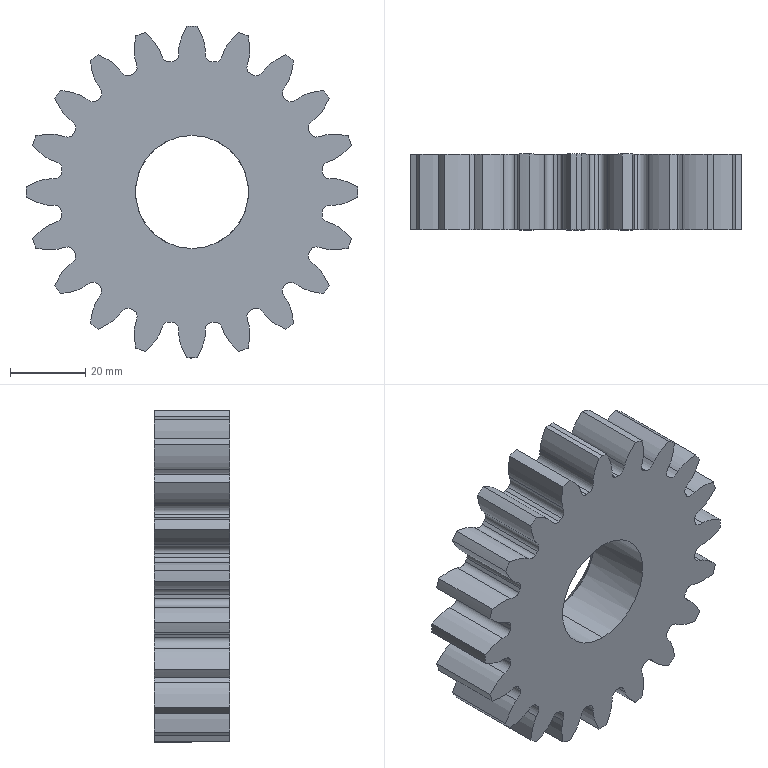Part | SolidWorks | features BaseBody 1 | 1 solid | 127 faces | box 88 x 20 x 88 mm | volume 84469 mm3 | spline 80 | cylinder 43 | cone 2 | plane 2 | commonest cylinder face diameters 88.007 x21 70 x20 30 x2